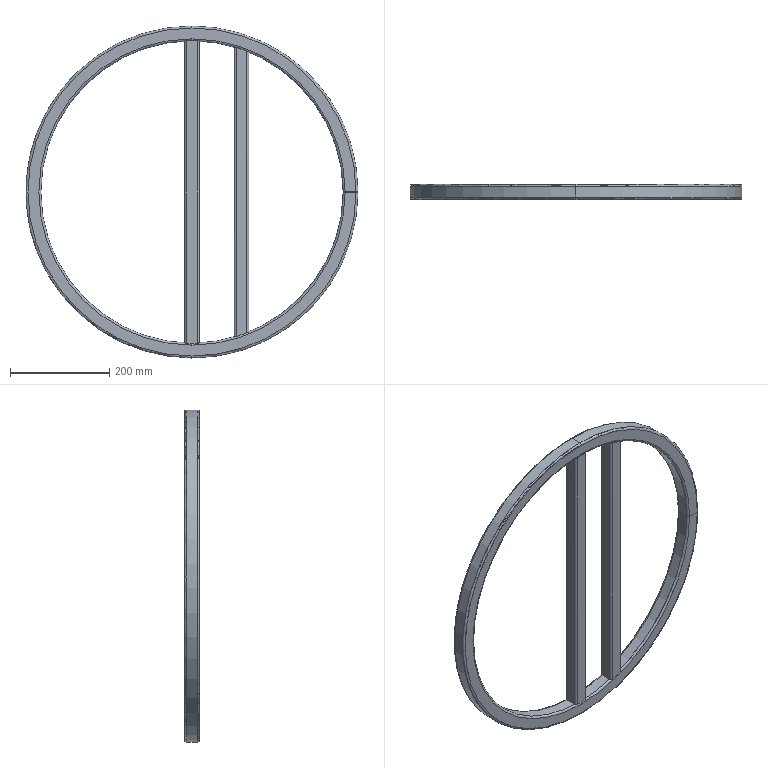Part | SolidWorks | features ICE 1, WeldMemberFeat 1, WeldmentFeature 1 | 3 solids | 79 faces | box 670 x 30 x 670 mm | volume 682937 mm3 | cylinder 33 | torus 24 | plane 22 | commonest cylinder face diameters 4 x8 8 x8 610 x8 614 x3 666 x3 670 x3